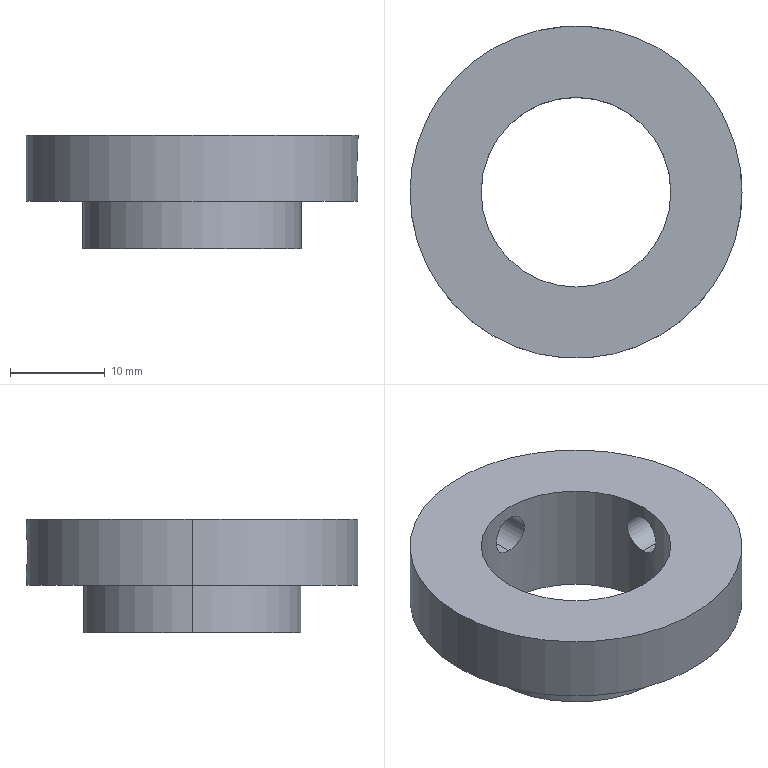Part | SolidWorks | features BaseBody 1 | 1 solid | 13 faces | box 35 x 35 x 12 mm | volume 4834 mm3 | cylinder 10 | plane 3 | commonest cylinder face diameters 4.2 x4 20 x2 23 x2 35 x2
STEP:
#1=CARTESIAN_POINT('',(10.,0.,6.4));
#2=VERTEX_POINT('',#1);
#3=CARTESIAN_POINT('',(10.,0.,10.6));
#4=VERTEX_POINT('',#3);
#5=CARTESIAN_POINT('',(10.,0.,6.4));
#6=CARTESIAN_POINT('',(10.,-0.1391,6.4));
#7=CARTESIAN_POINT('',(9.997,-0.2759,6.414));
#8=CARTESIAN_POINT('',(9.986,-0.5447,6.467));
#9=CARTESIAN_POINT('',(9.978,-0.6783,6.508));
#10=CARTESIAN_POINT('',(9.957,-0.9324,6.613));
#11=CARTESIAN_POINT('',(9.945,-1.053,6.678));
#12=CARTESIAN_POINT('',(9.918,-1.281,6.83));
#13=CARTESIAN_POINT('',(9.904,-1.388,6.919));
#14=CARTESIAN_POINT('',(9.86,-1.678,7.208));
#15=CARTESIAN_POINT('',(9.831,-1.834,7.442));
#16=CARTESIAN_POINT('',(9.8,-1.992,7.821));
#17=CARTESIAN_POINT('',(9.791,-2.032,7.953));
#18=CARTESIAN_POINT('',(9.78,-2.086,8.224));
#19=CARTESIAN_POINT('',(9.777,-2.1,8.361));
#20=CARTESIAN_POINT('',(9.777,-2.1,8.636));
#21=CARTESIAN_POINT('',(9.78,-2.086,8.775));
#22=CARTESIAN_POINT('',(9.791,-2.033,9.045));
#23=CARTESIAN_POINT('',(9.8,-1.993,9.176));
#24=CARTESIAN_POINT('',(9.831,-1.835,9.558));
#25=CARTESIAN_POINT('',(9.86,-1.681,9.789));
#26=CARTESIAN_POINT('',(9.904,-1.388,10.082));
#27=CARTESIAN_POINT('',(9.918,-1.283,10.168));
#28=CARTESIAN_POINT('',(9.945,-1.056,10.32));
#29=CARTESIAN_POINT('',(9.957,-0.9328,10.386));
#30=CARTESIAN_POINT('',(9.978,-0.6792,10.492));
#31=CARTESIAN_POINT('',(9.986,-0.5483,10.532));
#32=CARTESIAN_POINT('',(9.997,-0.2784,10.586));
#33=CARTESIAN_POINT('',(10.,-0.1391,10.6));
#34=CARTESIAN_POINT('',(10.,0.,10.6));
#35=B_SPLINE_CURVE_WITH_KNOTS('',3,(#5,#6,#7,#8,#9,#10,#11,#12,#13,#14,#15,#16,#17,#18,#19,#20,#21,#22,#23,#24,#25,#26,#27,#28,#29,#30,#31,#32,#33,#34),.UNSPECIFIED.,.F.,.F.,(4,2,2,2,2,2,2,2,2,2,2,2,2,2,4),(0.,0.0004114,0.0008228,0.001234,0.001646,0.002468,0.00288,0.003291,0.003702,0.004114,0.004937,0.005348,0.005759,0.006171,0.006582),.UNSPECIFIED.);
#36=EDGE_CURVE('',#2,#4,#35,.T.);
#37=ORIENTED_EDGE('',*,*,#36,.T.);
#38=CARTESIAN_POINT('',(17.5,0.,10.6));
#39=VERTEX_POINT('',#38);
#40=CARTESIAN_POINT('',(17.5,0.,10.6));
#41=DIRECTION('',(1.,0.,0.));
#42=VECTOR('',#41,1000.);
#43=LINE('',#40,#42);
#44=EDGE_CURVE('',#4,#39,#43,.T.);
#45=ORIENTED_EDGE('',*,*,#44,.T.);
#46=CARTESIAN_POINT('',(17.5,0.,6.4));
#47=VERTEX_POINT('',#46);
#48=CARTESIAN_POINT('',(17.5,0.,10.6));
#49=CARTESIAN_POINT('',(17.5,-0.1389,10.6));
#50=CARTESIAN_POINT('',(17.498,-0.2754,10.586));
#51=CARTESIAN_POINT('',(17.492,-0.5439,10.533));
#52=CARTESIAN_POINT('',(17.487,-0.6773,10.493));
#53=CARTESIAN_POINT('',(17.476,-0.9315,10.387));
#54=CARTESIAN_POINT('',(17.469,-1.052,10.323));
#55=CARTESIAN_POINT('',(17.453,-1.28,10.17));
#56=CARTESIAN_POINT('',(17.445,-1.388,10.082));
#57=CARTESIAN_POINT('',(17.42,-1.678,9.791));
#58=CARTESIAN_POINT('',(17.404,-1.835,9.557));
#59=CARTESIAN_POINT('',(17.38,-2.044,9.052));
#60=CARTESIAN_POINT('',(17.374,-2.1,8.776));
#61=CARTESIAN_POINT('',(17.374,-2.1,8.364));
#62=CARTESIAN_POINT('',(17.375,-2.086,8.225));
#63=CARTESIAN_POINT('',(17.382,-2.033,7.956));
#64=CARTESIAN_POINT('',(17.386,-1.993,7.825));
#65=CARTESIAN_POINT('',(17.398,-1.888,7.57));
#66=CARTESIAN_POINT('',(17.405,-1.822,7.448));
#67=CARTESIAN_POINT('',(17.42,-1.671,7.22));
#68=CARTESIAN_POINT('',(17.428,-1.584,7.114));
#69=CARTESIAN_POINT('',(17.445,-1.388,6.918));
#70=CARTESIAN_POINT('',(17.453,-1.282,6.831));
#71=CARTESIAN_POINT('',(17.469,-1.055,6.679));
#72=CARTESIAN_POINT('',(17.476,-0.9321,6.613));
#73=CARTESIAN_POINT('',(17.487,-0.678,6.508));
#74=CARTESIAN_POINT('',(17.492,-0.5471,6.468));
#75=CARTESIAN_POINT('',(17.498,-0.2778,6.414));
#76=CARTESIAN_POINT('',(17.5,-0.1389,6.4));
#77=CARTESIAN_POINT('',(17.5,0.,6.4));
#78=B_SPLINE_CURVE_WITH_KNOTS('',3,(#48,#49,#50,#51,#52,#53,#54,#55,#56,#57,#58,#59,#60,#61,#62,#63,#64,#65,#66,#67,#68,#69,#70,#71,#72,#73,#74,#75,#76,#77),.UNSPECIFIED.,.F.,.F.,(4,2,2,2,2,2,2,2,2,2,2,2,2,2,4),(0.,0.0004106,0.0008212,0.001232,0.001642,0.002464,0.003285,0.003696,0.004106,0.004517,0.004927,0.005338,0.005749,0.006159,0.00657),.UNSPECIFIED.);
#79=EDGE_CURVE('',#39,#47,#78,.T.);
#80=ORIENTED_EDGE('',*,*,#79,.T.);
#81=CARTESIAN_POINT('',(17.5,0.,6.4));
#82=DIRECTION('',(1.,0.,0.));
#83=VECTOR('',#82,1000.);
#84=LINE('',#81,#83);
#85=EDGE_CURVE('',#2,#47,#84,.T.);
#86=ORIENTED_EDGE('',*,*,#85,.F.);
#87=EDGE_LOOP('',(#37,#45,#80,#86));
#88=FACE_OUTER_BOUND('',#87,.T.);
#89=CARTESIAN_POINT('',(17.5,0.,8.5));
#90=DIRECTION('',(1.,0.,0.));
#91=DIRECTION('',(0.,0.,-1.));
#92=AXIS2_PLACEMENT_3D('',#89,#90,#91);
#93=CYLINDRICAL_SURFACE('',#92,2.1);
#94=ADVANCED_FACE('',(#88),#93,.F.);
#95=CARTESIAN_POINT('',(0.,10.,10.6));
#96=VERTEX_POINT('',#95);
#97=CARTESIAN_POINT('',(0.,10.,6.4));
#98=VERTEX_POINT('',#97);
#99=CARTESIAN_POINT('',(0.,10.,10.6));
#100=CARTESIAN_POINT('',(-0.1391,10.,10.6));
#101=CARTESIAN_POINT('',(-0.2759,9.997,10.586));
#102=CARTESIAN_POINT('',(-0.5447,9.986,10.533));
#103=CARTESIAN_POINT('',(-0.6783,9.978,10.492));
#104=CARTESIAN_POINT('',(-0.9324,9.957,10.387));
#105=CARTESIAN_POINT('',(-1.053,9.945,10.322));
#106=CARTESIAN_POINT('',(-1.281,9.918,10.17));
#107=CARTESIAN_POINT('',(-1.388,9.904,10.081));
#108=CARTESIAN_POINT('',(-1.678,9.86,9.792));
#109=CARTESIAN_POINT('',(-1.834,9.831,9.558));
#110=CARTESIAN_POINT('',(-1.992,9.8,9.179));
#111=CARTESIAN_POINT('',(-2.032,9.791,9.047));
#112=CARTESIAN_POINT('',(-2.086,9.78,8.776));
#113=CARTESIAN_POINT('',(-2.1,9.777,8.639));
#114=CARTESIAN_POINT('',(-2.1,9.777,8.364));
#115=CARTESIAN_POINT('',(-2.086,9.78,8.225));
#116=CARTESIAN_POINT('',(-2.033,9.791,7.955));
#117=CARTESIAN_POINT('',(-1.993,9.8,7.824));
#118=CARTESIAN_POINT('',(-1.835,9.831,7.442));
#119=CARTESIAN_POINT('',(-1.681,9.86,7.211));
#120=CARTESIAN_POINT('',(-1.388,9.904,6.918));
#121=CARTESIAN_POINT('',(-1.283,9.918,6.832));
#122=CARTESIAN_POINT('',(-1.056,9.945,6.68));
#123=CARTESIAN_POINT('',(-0.9328,9.957,6.614));
#124=CARTESIAN_POINT('',(-0.6792,9.978,6.508));
#125=CARTESIAN_POINT('',(-0.5483,9.986,6.468));
#126=CARTESIAN_POINT('',(-0.2784,9.997,6.414));
#127=CARTESIAN_POINT('',(-0.1391,10.,6.4));
#128=CARTESIAN_POINT('',(0.,10.,6.4));
#129=B_SPLINE_CURVE_WITH_KNOTS('',3,(#99,#100,#101,#102,#103,#104,#105,#106,#107,#108,#109,#110,#111,#112,#113,#114,#115,#116,#117,#118,#119,#120,#121,#122,#123,#124,#125,#126,#127,#128),.UNSPECIFIED.,.F.,.F.,(4,2,2,2,2,2,2,2,2,2,2,2,2,2,4),(0.,0.0004114,0.0008228,0.001234,0.001646,0.002468,0.00288,0.003291,0.003702,0.004114,0.004937,0.005348,0.005759,0.006171,0.006582),.UNSPECIFIED.);
#130=EDGE_CURVE('',#96,#98,#129,.T.);
#131=ORIENTED_EDGE('',*,*,#130,.T.);
#132=CARTESIAN_POINT('',(0.,17.5,6.4));
#133=VERTEX_POINT('',#132);
#134=CARTESIAN_POINT('',(0.,17.5,6.4));
#135=DIRECTION('',(0.,1.,0.));
#136=VECTOR('',#135,1000.);
#137=LINE('',#134,#136);
#138=EDGE_CURVE('',#98,#133,#137,.T.);
#139=ORIENTED_EDGE('',*,*,#138,.T.);
#140=CARTESIAN_POINT('',(0.,17.5,10.6));
#141=VERTEX_POINT('',#140);
#142=CARTESIAN_POINT('',(0.,17.5,6.4));
#143=CARTESIAN_POINT('',(-0.1389,17.5,6.4));
#144=CARTESIAN_POINT('',(-0.2754,17.498,6.414));
#145=CARTESIAN_POINT('',(-0.5439,17.492,6.467));
#146=CARTESIAN_POINT('',(-0.6773,17.487,6.507));
#147=CARTESIAN_POINT('',(-0.9315,17.476,6.613));
#148=CARTESIAN_POINT('',(-1.052,17.469,6.677));
#149=CARTESIAN_POINT('',(-1.28,17.453,6.83));
#150=CARTESIAN_POINT('',(-1.388,17.445,6.918));
#151=CARTESIAN_POINT('',(-1.678,17.42,7.209));
#152=CARTESIAN_POINT('',(-1.835,17.404,7.443));
#153=CARTESIAN_POINT('',(-2.044,17.38,7.948));
#154=CARTESIAN_POINT('',(-2.1,17.374,8.224));
#155=CARTESIAN_POINT('',(-2.1,17.374,8.636));
#156=CARTESIAN_POINT('',(-2.086,17.375,8.775));
#157=CARTESIAN_POINT('',(-2.033,17.382,9.044));
#158=CARTESIAN_POINT('',(-1.993,17.386,9.175));
#159=CARTESIAN_POINT('',(-1.888,17.398,9.43));
#160=CARTESIAN_POINT('',(-1.822,17.405,9.552));
#161=CARTESIAN_POINT('',(-1.671,17.42,9.78));
#162=CARTESIAN_POINT('',(-1.584,17.428,9.886));
#163=CARTESIAN_POINT('',(-1.388,17.445,10.082));
#164=CARTESIAN_POINT('',(-1.282,17.453,10.169));
#165=CARTESIAN_POINT('',(-1.055,17.469,10.321));
#166=CARTESIAN_POINT('',(-0.9321,17.476,10.387));
#167=CARTESIAN_POINT('',(-0.678,17.487,10.492));
#168=CARTESIAN_POINT('',(-0.5471,17.492,10.532));
#169=CARTESIAN_POINT('',(-0.2778,17.498,10.586));
#170=CARTESIAN_POINT('',(-0.1389,17.5,10.6));
#171=CARTESIAN_POINT('',(0.,17.5,10.6));
#172=B_SPLINE_CURVE_WITH_KNOTS('',3,(#142,#143,#144,#145,#146,#147,#148,#149,#150,#151,#152,#153,#154,#155,#156,#157,#158,#159,#160,#161,#162,#163,#164,#165,#166,#167,#168,#169,#170,#171),.UNSPECIFIED.,.F.,.F.,(4,2,2,2,2,2,2,2,2,2,2,2,2,2,4),(0.,0.0004106,0.0008212,0.001232,0.001642,0.002464,0.003285,0.003696,0.004106,0.004517,0.004927,0.005338,0.005749,0.006159,0.00657),.UNSPECIFIED.);
#173=EDGE_CURVE('',#133,#141,#172,.T.);
#174=ORIENTED_EDGE('',*,*,#173,.T.);
#175=CARTESIAN_POINT('',(0.,17.5,10.6));
#176=DIRECTION('',(0.,1.,0.));
#177=VECTOR('',#176,1000.);
#178=LINE('',#175,#177);
#179=EDGE_CURVE('',#96,#141,#178,.T.);
#180=ORIENTED_EDGE('',*,*,#179,.F.);
#181=EDGE_LOOP('',(#131,#139,#174,#180));
#182=FACE_OUTER_BOUND('',#181,.T.);
#183=CARTESIAN_POINT('',(0.,17.5,8.5));
#184=DIRECTION('',(0.,1.,0.));
#185=DIRECTION('',(0.,0.,1.));
#186=AXIS2_PLACEMENT_3D('',#183,#184,#185);
#187=CYLINDRICAL_SURFACE('',#186,2.1);
#188=ADVANCED_FACE('',(#182),#187,.F.);
#189=CARTESIAN_POINT('',(-11.5,0.,5.));
#190=VERTEX_POINT('',#189);
#191=CARTESIAN_POINT('',(11.5,0.,5.));
#192=VERTEX_POINT('',#191);
#193=CARTESIAN_POINT('',(0.,0.,5.));
#194=DIRECTION('',(0.,0.,-1.));
#195=DIRECTION('',(-1.,0.,0.));
#196=AXIS2_PLACEMENT_3D('',#193,#194,#195);
#197=CIRCLE('',#196,11.5);
#198=EDGE_CURVE('',#190,#192,#197,.T.);
#199=ORIENTED_EDGE('',*,*,#198,.T.);
#200=CARTESIAN_POINT('',(11.5,0.,0.));
#201=VERTEX_POINT('',#200);
#202=CARTESIAN_POINT('',(11.5,0.,0.));
#203=DIRECTION('',(0.,0.,-1.));
#204=VECTOR('',#203,1000.);
#205=LINE('',#202,#204);
#206=EDGE_CURVE('',#192,#201,#205,.T.);
#207=ORIENTED_EDGE('',*,*,#206,.T.);
#208=CARTESIAN_POINT('',(-11.5,0.,0.));
#209=VERTEX_POINT('',#208);
#210=CARTESIAN_POINT('',(0.,0.,0.));
#211=DIRECTION('',(0.,0.,-1.));
#212=DIRECTION('',(-1.,0.,0.));
#213=AXIS2_PLACEMENT_3D('',#210,#211,#212);
#214=CIRCLE('',#213,11.5);
#215=EDGE_CURVE('',#209,#201,#214,.T.);
#216=ORIENTED_EDGE('',*,*,#215,.F.);
#217=CARTESIAN_POINT('',(-11.5,0.,0.));
#218=DIRECTION('',(0.,0.,-1.));
#219=VECTOR('',#218,1000.);
#220=LINE('',#217,#219);
#221=EDGE_CURVE('',#190,#209,#220,.T.);
#222=ORIENTED_EDGE('',*,*,#221,.F.);
#223=EDGE_LOOP('',(#199,#207,#216,#222));
#224=FACE_OUTER_BOUND('',#223,.T.);
#225=CARTESIAN_POINT('',(0.,0.,0.));
#226=DIRECTION('',(0.,0.,-1.));
#227=DIRECTION('',(-1.,0.,0.));
#228=AXIS2_PLACEMENT_3D('',#225,#226,#227);
#229=CYLINDRICAL_SURFACE('',#228,11.5);
#230=ADVANCED_FACE('',(#224),#229,.T.);
#231=CARTESIAN_POINT('',(0.,17.5,10.6));
#232=CARTESIAN_POINT('',(0.1389,17.5,10.6));
#233=CARTESIAN_POINT('',(0.2754,17.498,10.586));
#234=CARTESIAN_POINT('',(0.5439,17.492,10.533));
#235=CARTESIAN_POINT('',(0.6773,17.487,10.493));
#236=CARTESIAN_POINT('',(0.9315,17.476,10.387));
#237=CARTESIAN_POINT('',(1.052,17.469,10.323));
#238=CARTESIAN_POINT('',(1.28,17.453,10.17));
#239=CARTESIAN_POINT('',(1.388,17.445,10.082));
#240=CARTESIAN_POINT('',(1.678,17.42,9.791));
#241=CARTESIAN_POINT('',(1.835,17.404,9.557));
#242=CARTESIAN_POINT('',(2.044,17.38,9.052));
#243=CARTESIAN_POINT('',(2.1,17.374,8.776));
#244=CARTESIAN_POINT('',(2.1,17.374,8.364));
#245=CARTESIAN_POINT('',(2.086,17.375,8.225));
#246=CARTESIAN_POINT('',(2.033,17.382,7.956));
#247=CARTESIAN_POINT('',(1.993,17.386,7.825));
#248=CARTESIAN_POINT('',(1.888,17.398,7.57));
#249=CARTESIAN_POINT('',(1.822,17.405,7.448));
#250=CARTESIAN_POINT('',(1.671,17.42,7.22));
#251=CARTESIAN_POINT('',(1.584,17.428,7.114));
#252=CARTESIAN_POINT('',(1.388,17.445,6.918));
#253=CARTESIAN_POINT('',(1.282,17.453,6.831));
#254=CARTESIAN_POINT('',(1.055,17.469,6.679));
#255=CARTESIAN_POINT('',(0.9321,17.476,6.613));
#256=CARTESIAN_POINT('',(0.678,17.487,6.508));
#257=CARTESIAN_POINT('',(0.5471,17.492,6.468));
#258=CARTESIAN_POINT('',(0.2778,17.498,6.414));
#259=CARTESIAN_POINT('',(0.1389,17.5,6.4));
#260=CARTESIAN_POINT('',(0.,17.5,6.4));
#261=B_SPLINE_CURVE_WITH_KNOTS('',3,(#231,#232,#233,#234,#235,#236,#237,#238,#239,#240,#241,#242,#243,#244,#245,#246,#247,#248,#249,#250,#251,#252,#253,#254,#255,#256,#257,#258,#259,#260),.UNSPECIFIED.,.F.,.F.,(4,2,2,2,2,2,2,2,2,2,2,2,2,2,4),(0.00657,0.006981,0.007391,0.007802,0.008212,0.009034,0.009855,0.01027,0.01068,0.01109,0.0115,0.01191,0.01232,0.01273,0.01314),.UNSPECIFIED.);
#262=EDGE_CURVE('',#141,#133,#261,.T.);
#263=ORIENTED_EDGE('',*,*,#262,.F.);
#264=ORIENTED_EDGE('',*,*,#173,.F.);
#265=EDGE_LOOP('',(#263,#264));
#266=FACE_BOUND('',#265,.T.);
#267=CARTESIAN_POINT('',(-17.5,0.,12.));
#268=VERTEX_POINT('',#267);
#269=CARTESIAN_POINT('',(17.5,0.,12.));
#270=VERTEX_POINT('',#269);
#271=CARTESIAN_POINT('',(0.,0.,12.));
#272=DIRECTION('',(0.,0.,-1.));
#273=DIRECTION('',(-1.,0.,0.));
#274=AXIS2_PLACEMENT_3D('',#271,#272,#273);
#275=CIRCLE('',#274,17.5);
#276=EDGE_CURVE('',#268,#270,#275,.T.);
#277=ORIENTED_EDGE('',*,*,#276,.T.);
#278=CARTESIAN_POINT('',(17.5,0.,0.));
#279=DIRECTION('',(0.,0.,-1.));
#280=VECTOR('',#279,1000.);
#281=LINE('',#278,#280);
#282=EDGE_CURVE('',#270,#39,#281,.T.);
#283=ORIENTED_EDGE('',*,*,#282,.T.);
#284=CARTESIAN_POINT('',(17.5,0.,6.4));
#285=CARTESIAN_POINT('',(17.5,0.1389,6.4));
#286=CARTESIAN_POINT('',(17.498,0.2754,6.414));
#287=CARTESIAN_POINT('',(17.492,0.5439,6.467));
#288=CARTESIAN_POINT('',(17.487,0.6773,6.507));
#289=CARTESIAN_POINT('',(17.476,0.9315,6.613));
#290=CARTESIAN_POINT('',(17.469,1.052,6.677));
#291=CARTESIAN_POINT('',(17.453,1.28,6.83));
#292=CARTESIAN_POINT('',(17.445,1.388,6.918));
#293=CARTESIAN_POINT('',(17.42,1.678,7.209));
#294=CARTESIAN_POINT('',(17.404,1.835,7.443));
#295=CARTESIAN_POINT('',(17.38,2.044,7.948));
#296=CARTESIAN_POINT('',(17.374,2.1,8.224));
#297=CARTESIAN_POINT('',(17.374,2.1,8.636));
#298=CARTESIAN_POINT('',(17.375,2.086,8.775));
#299=CARTESIAN_POINT('',(17.382,2.033,9.044));
#300=CARTESIAN_POINT('',(17.386,1.993,9.175));
#301=CARTESIAN_POINT('',(17.398,1.888,9.43));
#302=CARTESIAN_POINT('',(17.405,1.822,9.552));
#303=CARTESIAN_POINT('',(17.42,1.671,9.78));
#304=CARTESIAN_POINT('',(17.428,1.584,9.886));
#305=CARTESIAN_POINT('',(17.445,1.388,10.082));
#306=CARTESIAN_POINT('',(17.453,1.282,10.169));
#307=CARTESIAN_POINT('',(17.469,1.055,10.321));
#308=CARTESIAN_POINT('',(17.476,0.9321,10.387));
#309=CARTESIAN_POINT('',(17.487,0.678,10.492));
#310=CARTESIAN_POINT('',(17.492,0.5471,10.532));
#311=CARTESIAN_POINT('',(17.498,0.2778,10.586));
#312=CARTESIAN_POINT('',(17.5,0.1389,10.6));
#313=CARTESIAN_POINT('',(17.5,0.,10.6));
#314=B_SPLINE_CURVE_WITH_KNOTS('',3,(#284,#285,#286,#287,#288,#289,#290,#291,#292,#293,#294,#295,#296,#297,#298,#299,#300,#301,#302,#303,#304,#305,#306,#307,#308,#309,#310,#311,#312,#313),.UNSPECIFIED.,.F.,.F.,(4,2,2,2,2,2,2,2,2,2,2,2,2,2,4),(0.00657,0.006981,0.007391,0.007802,0.008212,0.009034,0.009855,0.01027,0.01068,0.01109,0.0115,0.01191,0.01232,0.01273,0.01314),.UNSPECIFIED.);
#315=EDGE_CURVE('',#47,#39,#314,.T.);
#316=ORIENTED_EDGE('',*,*,#315,.F.);
#317=CARTESIAN_POINT('',(17.5,0.,5.));
#318=VERTEX_POINT('',#317);
#319=CARTESIAN_POINT('',(17.5,0.,0.));
#320=DIRECTION('',(0.,0.,-1.));
#321=VECTOR('',#320,1000.);
#322=LINE('',#319,#321);
#323=EDGE_CURVE('',#47,#318,#322,.T.);
#324=ORIENTED_EDGE('',*,*,#323,.T.);
#325=CARTESIAN_POINT('',(-17.5,0.,5.));
#326=VERTEX_POINT('',#325);
#327=CARTESIAN_POINT('',(0.,0.,5.));
#328=DIRECTION('',(0.,0.,-1.));
#329=DIRECTION('',(-1.,0.,0.));
#330=AXIS2_PLACEMENT_3D('',#327,#328,#329);
#331=CIRCLE('',#330,17.5);
#332=EDGE_CURVE('',#326,#318,#331,.T.);
#333=ORIENTED_EDGE('',*,*,#332,.F.);
#334=CARTESIAN_POINT('',(-17.5,0.,0.));
#335=DIRECTION('',(0.,0.,-1.));
#336=VECTOR('',#335,1000.);
#337=LINE('',#334,#336);
#338=EDGE_CURVE('',#268,#326,#337,.T.);
#339=ORIENTED_EDGE('',*,*,#338,.F.);
#340=EDGE_LOOP('',(#277,#283,#316,#324,#333,#339));
#341=FACE_OUTER_BOUND('',#340,.T.);
#342=CARTESIAN_POINT('',(0.,0.,0.));
#343=DIRECTION('',(0.,0.,-1.));
#344=DIRECTION('',(-1.,0.,0.));
#345=AXIS2_PLACEMENT_3D('',#342,#343,#344);
#346=CYLINDRICAL_SURFACE('',#345,17.5);
#347=ADVANCED_FACE('',(#266,#341),#346,.T.);
#348=CARTESIAN_POINT('',(10.,0.,12.));
#349=VERTEX_POINT('',#348);
#350=CARTESIAN_POINT('',(-10.,0.,12.));
#351=VERTEX_POINT('',#350);
#352=CARTESIAN_POINT('',(0.,0.,12.));
#353=DIRECTION('',(0.,0.,-1.));
#354=DIRECTION('',(-1.,0.,0.));
#355=AXIS2_PLACEMENT_3D('',#352,#353,#354);
#356=CIRCLE('',#355,10.);
#357=EDGE_CURVE('',#349,#351,#356,.T.);
#358=ORIENTED_EDGE('',*,*,#357,.F.);
#359=CARTESIAN_POINT('',(10.,0.,0.));
#360=DIRECTION('',(0.,0.,-1.));
#361=VECTOR('',#360,1000.);
#362=LINE('',#359,#361);
#363=EDGE_CURVE('',#349,#4,#362,.T.);
#364=ORIENTED_EDGE('',*,*,#363,.T.);
#365=ORIENTED_EDGE('',*,*,#36,.F.);
#366=CARTESIAN_POINT('',(10.,0.,0.));
#367=VERTEX_POINT('',#366);
#368=CARTESIAN_POINT('',(10.,0.,0.));
#369=DIRECTION('',(0.,0.,-1.));
#370=VECTOR('',#369,1000.);
#371=LINE('',#368,#370);
#372=EDGE_CURVE('',#2,#367,#371,.T.);
#373=ORIENTED_EDGE('',*,*,#372,.T.);
#374=CARTESIAN_POINT('',(-10.,0.,0.));
#375=VERTEX_POINT('',#374);
#376=CARTESIAN_POINT('',(0.,0.,0.));
#377=DIRECTION('',(0.,0.,-1.));
#378=DIRECTION('',(-1.,0.,0.));
#379=AXIS2_PLACEMENT_3D('',#376,#377,#378);
#380=CIRCLE('',#379,10.);
#381=EDGE_CURVE('',#367,#375,#380,.T.);
#382=ORIENTED_EDGE('',*,*,#381,.T.);
#383=CARTESIAN_POINT('',(-10.,0.,0.));
#384=DIRECTION('',(0.,0.,-1.));
#385=VECTOR('',#384,1000.);
#386=LINE('',#383,#385);
#387=EDGE_CURVE('',#351,#375,#386,.T.);
#388=ORIENTED_EDGE('',*,*,#387,.F.);
#389=EDGE_LOOP('',(#358,#364,#365,#373,#382,#388));
#390=FACE_OUTER_BOUND('',#389,.T.);
#391=CARTESIAN_POINT('',(0.,0.,0.));
#392=DIRECTION('',(0.,0.,-1.));
#393=DIRECTION('',(-1.,0.,0.));
#394=AXIS2_PLACEMENT_3D('',#391,#392,#393);
#395=CYLINDRICAL_SURFACE('',#394,10.);
#396=ADVANCED_FACE('',(#390),#395,.F.);
#397=ORIENTED_EDGE('',*,*,#198,.F.);
#398=CARTESIAN_POINT('',(0.,0.,5.));
#399=DIRECTION('',(0.,0.,-1.));
#400=DIRECTION('',(-1.,0.,0.));
#401=AXIS2_PLACEMENT_3D('',#398,#399,#400);
#402=CIRCLE('',#401,11.5);
#403=EDGE_CURVE('',#192,#190,#402,.T.);
#404=ORIENTED_EDGE('',*,*,#403,.F.);
#405=EDGE_LOOP('',(#397,#404));
#406=FACE_BOUND('',#405,.T.);
#407=ORIENTED_EDGE('',*,*,#332,.T.);
#408=CARTESIAN_POINT('',(0.,0.,5.));
#409=DIRECTION('',(0.,0.,-1.));
#410=DIRECTION('',(-1.,0.,0.));
#411=AXIS2_PLACEMENT_3D('',#408,#409,#410);
#412=CIRCLE('',#411,17.5);
#413=EDGE_CURVE('',#318,#326,#412,.T.);
#414=ORIENTED_EDGE('',*,*,#413,.T.);
#415=EDGE_LOOP('',(#407,#414));
#416=FACE_OUTER_BOUND('',#415,.T.);
#417=CARTESIAN_POINT('',(0.,17.5,5.));
#418=DIRECTION('',(0.,0.,-1.));
#419=DIRECTION('',(0.,-1.,0.));
#420=AXIS2_PLACEMENT_3D('',#417,#418,#419);
#421=PLANE('',#420);
#422=ADVANCED_FACE('',(#406,#416),#421,.T.);
#423=CARTESIAN_POINT('',(0.,0.,12.));
#424=DIRECTION('',(0.,0.,-1.));
#425=DIRECTION('',(-1.,0.,0.));
#426=AXIS2_PLACEMENT_3D('',#423,#424,#425);
#427=CIRCLE('',#426,10.);
#428=EDGE_CURVE('',#351,#349,#427,.T.);
#429=ORIENTED_EDGE('',*,*,#428,.T.);
#430=ORIENTED_EDGE('',*,*,#357,.T.);
#431=EDGE_LOOP('',(#429,#430));
#432=FACE_BOUND('',#431,.T.);
#433=ORIENTED_EDGE('',*,*,#276,.F.);
#434=CARTESIAN_POINT('',(0.,0.,12.));
#435=DIRECTION('',(0.,0.,-1.));
#436=DIRECTION('',(-1.,0.,0.));
#437=AXIS2_PLACEMENT_3D('',#434,#435,#436);
#438=CIRCLE('',#437,17.5);
#439=EDGE_CURVE('',#270,#268,#438,.T.);
#440=ORIENTED_EDGE('',*,*,#439,.F.);
#441=EDGE_LOOP('',(#433,#440));
#442=FACE_OUTER_BOUND('',#441,.T.);
#443=CARTESIAN_POINT('',(0.,10.,12.));
#444=DIRECTION('',(0.,0.,1.));
#445=DIRECTION('',(1.,0.,0.));
#446=AXIS2_PLACEMENT_3D('',#443,#444,#445);
#447=PLANE('',#446);
#448=ADVANCED_FACE('',(#432,#442),#447,.T.);
#449=CARTESIAN_POINT('',(0.,0.,0.));
#450=DIRECTION('',(0.,0.,-1.));
#451=DIRECTION('',(-1.,0.,0.));
#452=AXIS2_PLACEMENT_3D('',#449,#450,#451);
#453=CIRCLE('',#452,10.);
#454=EDGE_CURVE('',#375,#367,#453,.T.);
#455=ORIENTED_EDGE('',*,*,#454,.F.);
#456=ORIENTED_EDGE('',*,*,#381,.F.);
#457=EDGE_LOOP('',(#455,#456));
#458=FACE_BOUND('',#457,.T.);
#459=ORIENTED_EDGE('',*,*,#215,.T.);
#460=CARTESIAN_POINT('',(0.,0.,0.));
#461=DIRECTION('',(0.,0.,-1.));
#462=DIRECTION('',(-1.,0.,0.));
#463=AXIS2_PLACEMENT_3D('',#460,#461,#462);
#464=CIRCLE('',#463,11.5);
#465=EDGE_CURVE('',#201,#209,#464,.T.);
#466=ORIENTED_EDGE('',*,*,#465,.T.);
#467=EDGE_LOOP('',(#459,#466));
#468=FACE_OUTER_BOUND('',#467,.T.);
#469=CARTESIAN_POINT('',(0.,11.5,0.));
#470=DIRECTION('',(0.,0.,-1.));
#471=DIRECTION('',(0.,-1.,0.));
#472=AXIS2_PLACEMENT_3D('',#469,#470,#471);
#473=PLANE('',#472);
#474=ADVANCED_FACE('',(#458,#468),#473,.T.);
#475=ORIENTED_EDGE('',*,*,#363,.F.);
#476=ORIENTED_EDGE('',*,*,#428,.F.);
#477=ORIENTED_EDGE('',*,*,#387,.T.);
#478=ORIENTED_EDGE('',*,*,#454,.T.);
#479=ORIENTED_EDGE('',*,*,#372,.F.);
#480=CARTESIAN_POINT('',(10.,0.,10.6));
#481=CARTESIAN_POINT('',(10.,0.1391,10.6));
#482=CARTESIAN_POINT('',(9.997,0.2759,10.586));
#483=CARTESIAN_POINT('',(9.986,0.5447,10.533));
#484=CARTESIAN_POINT('',(9.978,0.6783,10.492));
#485=CARTESIAN_POINT('',(9.957,0.9324,10.387));
#486=CARTESIAN_POINT('',(9.945,1.053,10.322));
#487=CARTESIAN_POINT('',(9.918,1.281,10.17));
#488=CARTESIAN_POINT('',(9.904,1.388,10.081));
#489=CARTESIAN_POINT('',(9.86,1.678,9.792));
#490=CARTESIAN_POINT('',(9.831,1.834,9.558));
#491=CARTESIAN_POINT('',(9.8,1.992,9.179));
#492=CARTESIAN_POINT('',(9.791,2.032,9.047));
#493=CARTESIAN_POINT('',(9.78,2.086,8.776));
#494=CARTESIAN_POINT('',(9.777,2.1,8.639));
#495=CARTESIAN_POINT('',(9.777,2.1,8.364));
#496=CARTESIAN_POINT('',(9.78,2.086,8.225));
#497=CARTESIAN_POINT('',(9.791,2.033,7.955));
#498=CARTESIAN_POINT('',(9.8,1.993,7.824));
#499=CARTESIAN_POINT('',(9.831,1.835,7.442));
#500=CARTESIAN_POINT('',(9.86,1.681,7.211));
#501=CARTESIAN_POINT('',(9.904,1.388,6.918));
#502=CARTESIAN_POINT('',(9.918,1.283,6.832));
#503=CARTESIAN_POINT('',(9.945,1.056,6.68));
#504=CARTESIAN_POINT('',(9.957,0.9328,6.614));
#505=CARTESIAN_POINT('',(9.978,0.6792,6.508));
#506=CARTESIAN_POINT('',(9.986,0.5483,6.468));
#507=CARTESIAN_POINT('',(9.997,0.2784,6.414));
#508=CARTESIAN_POINT('',(10.,0.1391,6.4));
#509=CARTESIAN_POINT('',(10.,0.,6.4));
#510=B_SPLINE_CURVE_WITH_KNOTS('',3,(#480,#481,#482,#483,#484,#485,#486,#487,#488,#489,#490,#491,#492,#493,#494,#495,#496,#497,#498,#499,#500,#501,#502,#503,#504,#505,#506,#507,#508,#509),.UNSPECIFIED.,.F.,.F.,(4,2,2,2,2,2,2,2,2,2,2,2,2,2,4),(0.006582,0.006993,0.007405,0.007816,0.008228,0.00905,0.009462,0.009873,0.01028,0.0107,0.01152,0.01193,0.01234,0.01275,0.01316),.UNSPECIFIED.);
#511=EDGE_CURVE('',#4,#2,#510,.T.);
#512=ORIENTED_EDGE('',*,*,#511,.F.);
#513=EDGE_LOOP('',(#475,#476,#477,#478,#479,#512));
#514=FACE_OUTER_BOUND('',#513,.T.);
#515=ORIENTED_EDGE('',*,*,#130,.F.);
#516=CARTESIAN_POINT('',(0.,10.,6.4));
#517=CARTESIAN_POINT('',(0.1391,10.,6.4));
#518=CARTESIAN_POINT('',(0.2759,9.997,6.414));
#519=CARTESIAN_POINT('',(0.5447,9.986,6.467));
#520=CARTESIAN_POINT('',(0.6783,9.978,6.508));
#521=CARTESIAN_POINT('',(0.9324,9.957,6.613));
#522=CARTESIAN_POINT('',(1.053,9.945,6.678));
#523=CARTESIAN_POINT('',(1.281,9.918,6.83));
#524=CARTESIAN_POINT('',(1.388,9.904,6.919));
#525=CARTESIAN_POINT('',(1.678,9.86,7.208));
#526=CARTESIAN_POINT('',(1.834,9.831,7.442));
#527=CARTESIAN_POINT('',(1.992,9.8,7.821));
#528=CARTESIAN_POINT('',(2.032,9.791,7.953));
#529=CARTESIAN_POINT('',(2.086,9.78,8.224));
#530=CARTESIAN_POINT('',(2.1,9.777,8.361));
#531=CARTESIAN_POINT('',(2.1,9.777,8.636));
#532=CARTESIAN_POINT('',(2.086,9.78,8.775));
#533=CARTESIAN_POINT('',(2.033,9.791,9.045));
#534=CARTESIAN_POINT('',(1.993,9.8,9.176));
#535=CARTESIAN_POINT('',(1.835,9.831,9.558));
#536=CARTESIAN_POINT('',(1.681,9.86,9.789));
#537=CARTESIAN_POINT('',(1.388,9.904,10.082));
#538=CARTESIAN_POINT('',(1.283,9.918,10.168));
#539=CARTESIAN_POINT('',(1.056,9.945,10.32));
#540=CARTESIAN_POINT('',(0.9328,9.957,10.386));
#541=CARTESIAN_POINT('',(0.6792,9.978,10.492));
#542=CARTESIAN_POINT('',(0.5483,9.986,10.532));
#543=CARTESIAN_POINT('',(0.2784,9.997,10.586));
#544=CARTESIAN_POINT('',(0.1391,10.,10.6));
#545=CARTESIAN_POINT('',(0.,10.,10.6));
#546=B_SPLINE_CURVE_WITH_KNOTS('',3,(#516,#517,#518,#519,#520,#521,#522,#523,#524,#525,#526,#527,#528,#529,#530,#531,#532,#533,#534,#535,#536,#537,#538,#539,#540,#541,#542,#543,#544,#545),.UNSPECIFIED.,.F.,.F.,(4,2,2,2,2,2,2,2,2,2,2,2,2,2,4),(0.006582,0.006993,0.007405,0.007816,0.008228,0.00905,0.009462,0.009873,0.01028,0.0107,0.01152,0.01193,0.01234,0.01275,0.01316),.UNSPECIFIED.);
#547=EDGE_CURVE('',#98,#96,#546,.T.);
#548=ORIENTED_EDGE('',*,*,#547,.F.);
#549=EDGE_LOOP('',(#515,#548));
#550=FACE_BOUND('',#549,.T.);
#551=CARTESIAN_POINT('',(0.,0.,0.));
#552=DIRECTION('',(0.,0.,-1.));
#553=DIRECTION('',(-1.,0.,0.));
#554=AXIS2_PLACEMENT_3D('',#551,#552,#553);
#555=CYLINDRICAL_SURFACE('',#554,10.);
#556=ADVANCED_FACE('',(#514,#550),#555,.F.);
#557=ORIENTED_EDGE('',*,*,#282,.F.);
#558=ORIENTED_EDGE('',*,*,#439,.T.);
#559=ORIENTED_EDGE('',*,*,#338,.T.);
#560=ORIENTED_EDGE('',*,*,#413,.F.);
#561=ORIENTED_EDGE('',*,*,#323,.F.);
#562=ORIENTED_EDGE('',*,*,#79,.F.);
#563=EDGE_LOOP('',(#557,#558,#559,#560,#561,#562));
#564=FACE_OUTER_BOUND('',#563,.T.);
#565=CARTESIAN_POINT('',(0.,0.,0.));
#566=DIRECTION('',(0.,0.,-1.));
#567=DIRECTION('',(-1.,0.,0.));
#568=AXIS2_PLACEMENT_3D('',#565,#566,#567);
#569=CYLINDRICAL_SURFACE('',#568,17.5);
#570=ADVANCED_FACE('',(#564),#569,.T.);
#571=ORIENTED_EDGE('',*,*,#206,.F.);
#572=ORIENTED_EDGE('',*,*,#403,.T.);
#573=ORIENTED_EDGE('',*,*,#221,.T.);
#574=ORIENTED_EDGE('',*,*,#465,.F.);
#575=EDGE_LOOP('',(#571,#572,#573,#574));
#576=FACE_OUTER_BOUND('',#575,.T.);
#577=CARTESIAN_POINT('',(0.,0.,0.));
#578=DIRECTION('',(0.,0.,-1.));
#579=DIRECTION('',(-1.,0.,0.));
#580=AXIS2_PLACEMENT_3D('',#577,#578,#579);
#581=CYLINDRICAL_SURFACE('',#580,11.5);
#582=ADVANCED_FACE('',(#576),#581,.T.);
#583=ORIENTED_EDGE('',*,*,#138,.F.);
#584=ORIENTED_EDGE('',*,*,#547,.T.);
#585=ORIENTED_EDGE('',*,*,#179,.T.);
#586=ORIENTED_EDGE('',*,*,#262,.T.);
#587=EDGE_LOOP('',(#583,#584,#585,#586));
#588=FACE_OUTER_BOUND('',#587,.T.);
#589=CARTESIAN_POINT('',(0.,17.5,8.5));
#590=DIRECTION('',(0.,1.,0.));
#591=DIRECTION('',(0.,0.,1.));
#592=AXIS2_PLACEMENT_3D('',#589,#590,#591);
#593=CYLINDRICAL_SURFACE('',#592,2.1);
#594=ADVANCED_FACE('',(#588),#593,.F.);
#595=ORIENTED_EDGE('',*,*,#44,.F.);
#596=ORIENTED_EDGE('',*,*,#511,.T.);
#597=ORIENTED_EDGE('',*,*,#85,.T.);
#598=ORIENTED_EDGE('',*,*,#315,.T.);
#599=EDGE_LOOP('',(#595,#596,#597,#598));
#600=FACE_OUTER_BOUND('',#599,.T.);
#601=CARTESIAN_POINT('',(17.5,0.,8.5));
#602=DIRECTION('',(1.,0.,0.));
#603=DIRECTION('',(0.,0.,-1.));
#604=AXIS2_PLACEMENT_3D('',#601,#602,#603);
#605=CYLINDRICAL_SURFACE('',#604,2.1);
#606=ADVANCED_FACE('',(#600),#605,.F.);
#607=CLOSED_SHELL('',(#94,#188,#230,#347,#396,#422,#448,#474,#556,#570,#582,#594,#606));
#608=MANIFOLD_SOLID_BREP('',#607);
#609=CARTESIAN_POINT('',(0.,0.,0.));
#610=DIRECTION('',(0.,0.,1.));
#611=DIRECTION('',(1.,0.,0.));
#612=AXIS2_PLACEMENT_3D('',#609,#610,#611);
#613=(LENGTH_UNIT()NAMED_UNIT(*)SI_UNIT(.MILLI.,.METRE.));
#614=UNCERTAINTY_MEASURE_WITH_UNIT(LENGTH_MEASURE(0.00001),#613,'','');
#615=(NAMED_UNIT(*)PLANE_ANGLE_UNIT()SI_UNIT($,.RADIAN.));
#616=(NAMED_UNIT(*)SI_UNIT($,.STERADIAN.)SOLID_ANGLE_UNIT());
#617=(GEOMETRIC_REPRESENTATION_CONTEXT(3)GLOBAL_UNCERTAINTY_ASSIGNED_CONTEXT((#614))GLOBAL_UNIT_ASSIGNED_CONTEXT((#613,#615,#616))REPRESENTATION_CONTEXT('',''));
#618=ADVANCED_BREP_SHAPE_REPRESENTATION('',(#608,#612),#617);